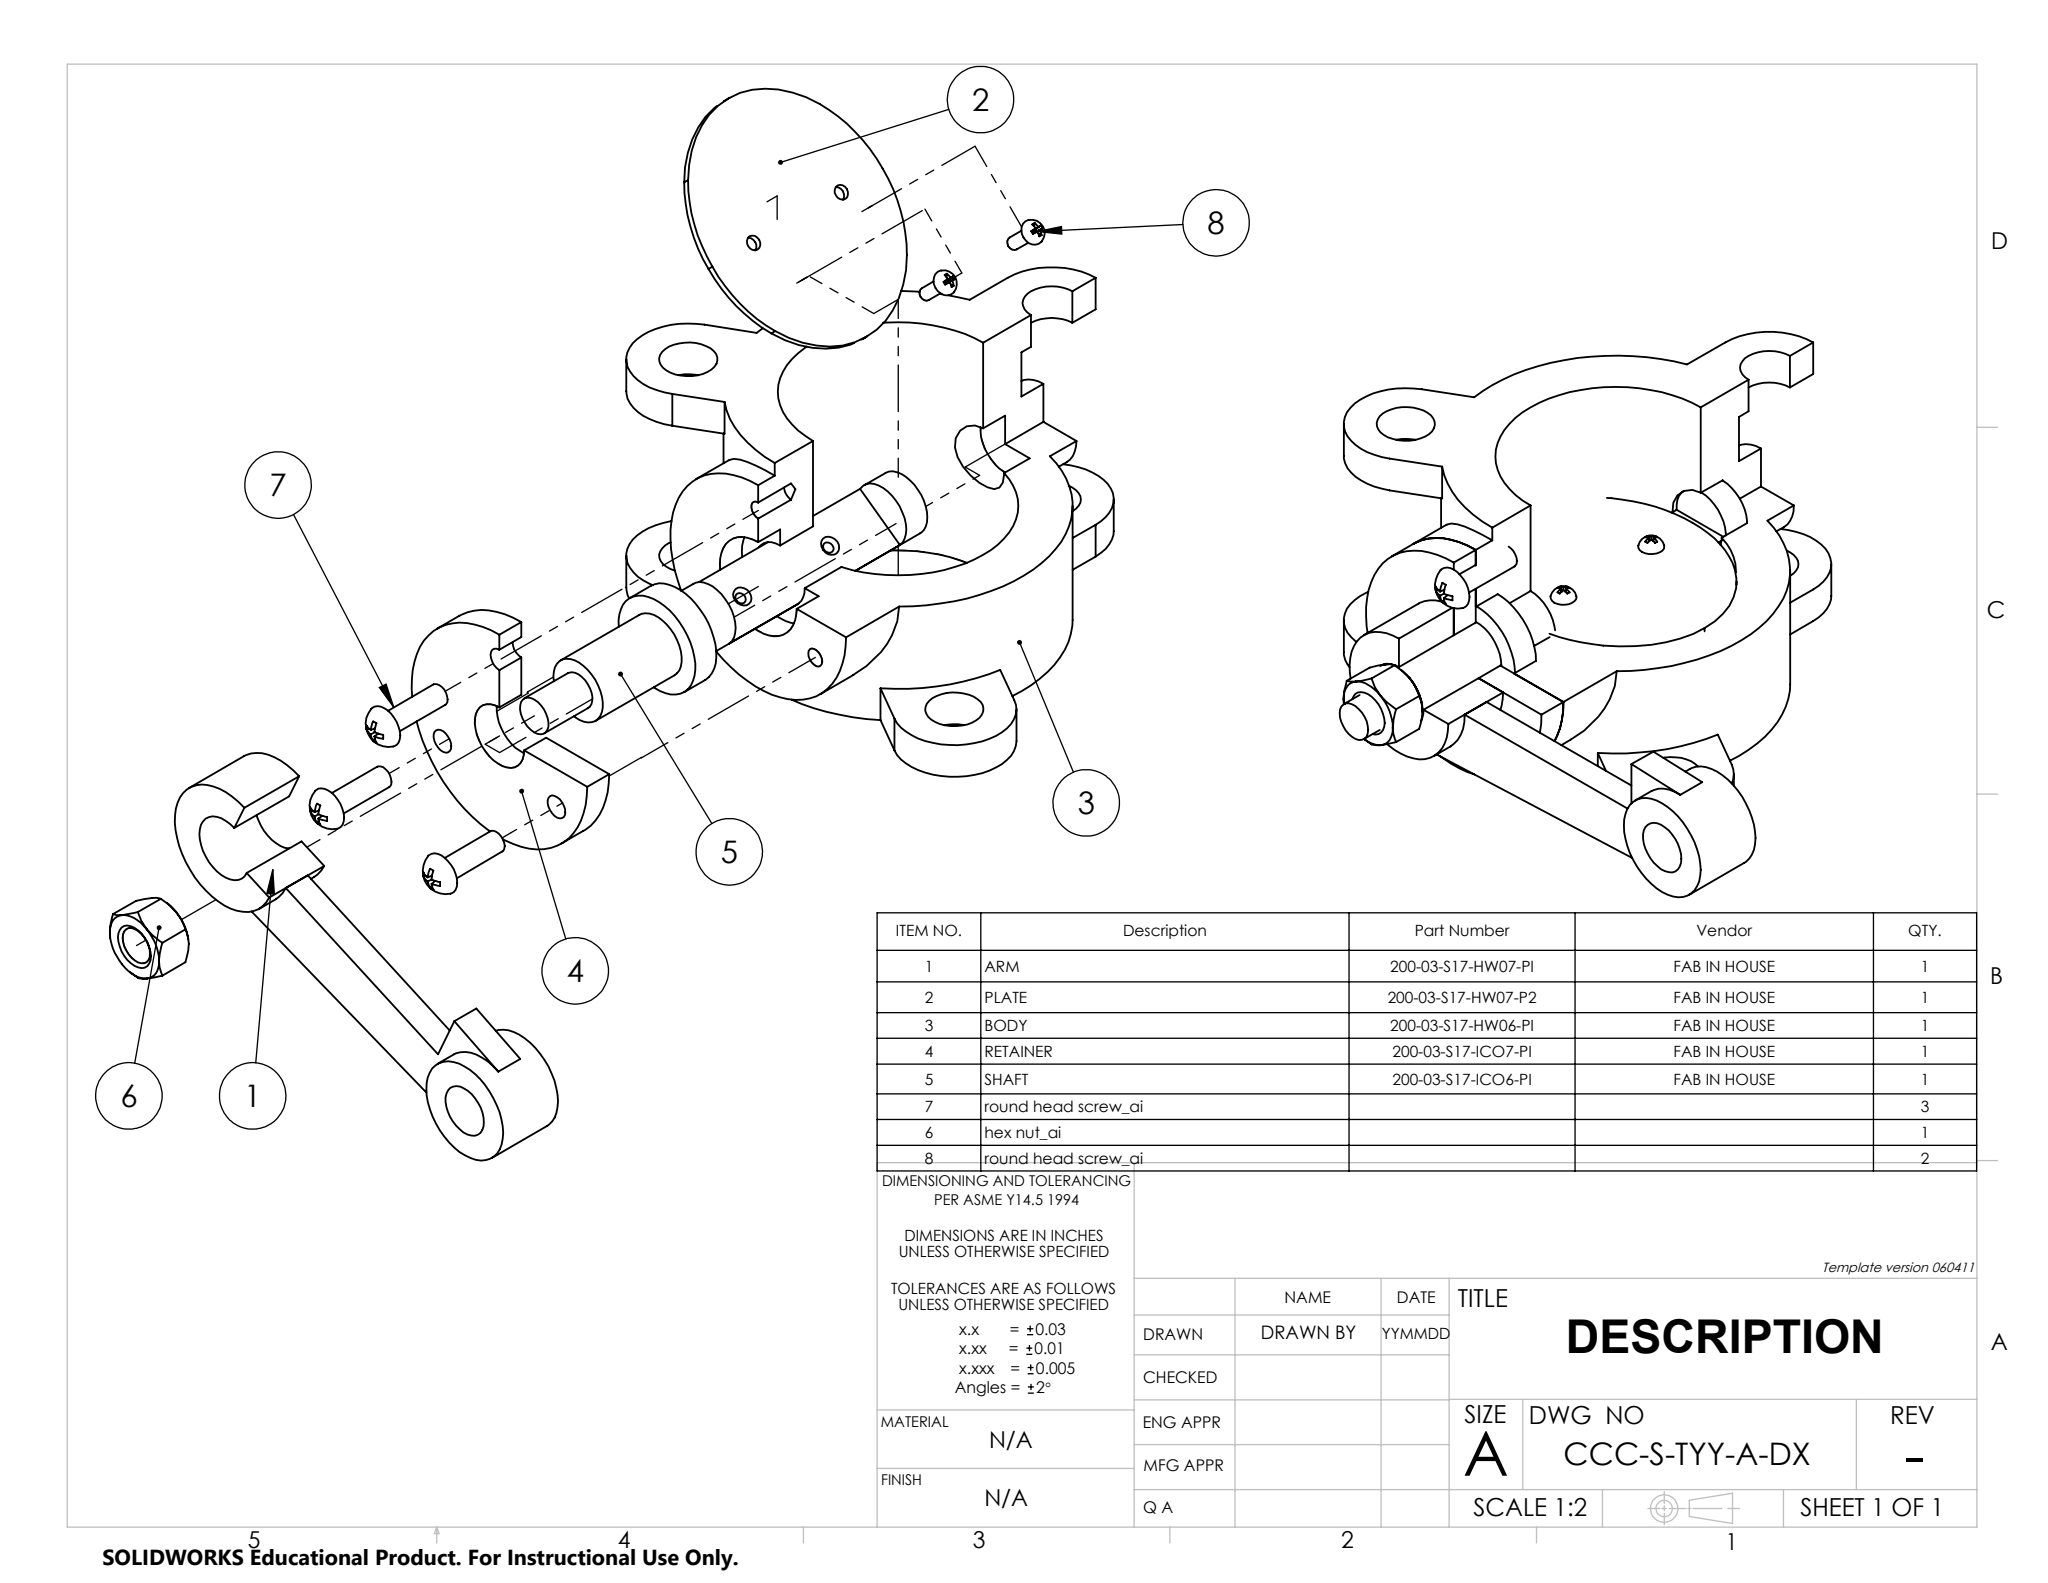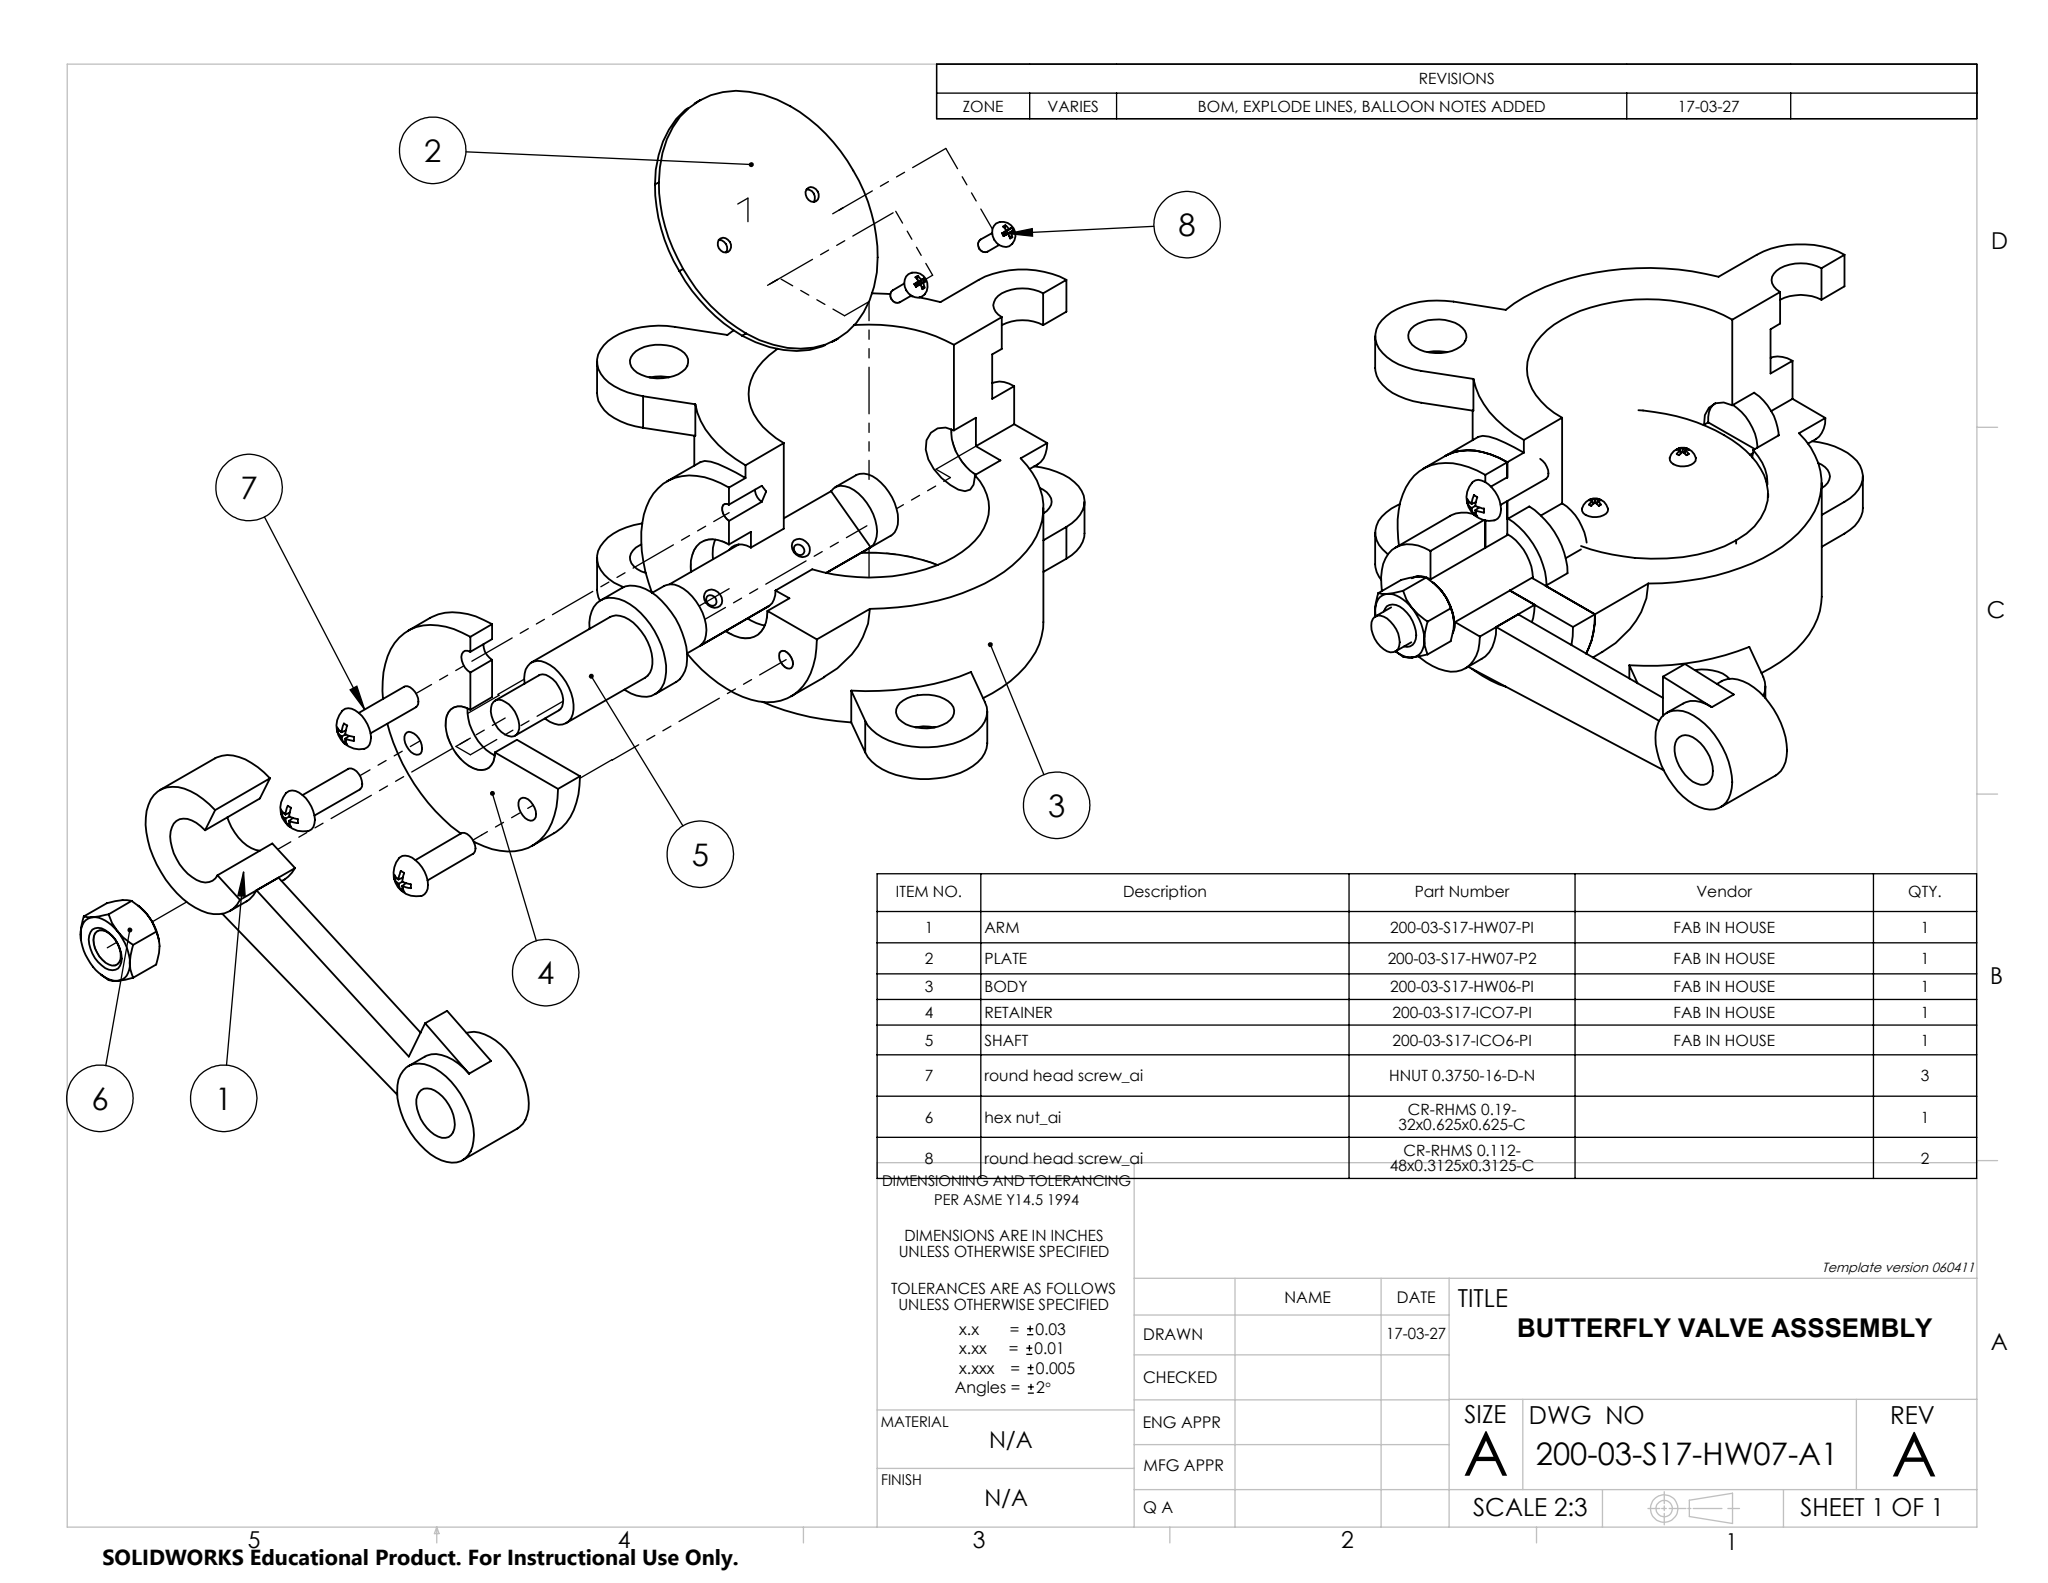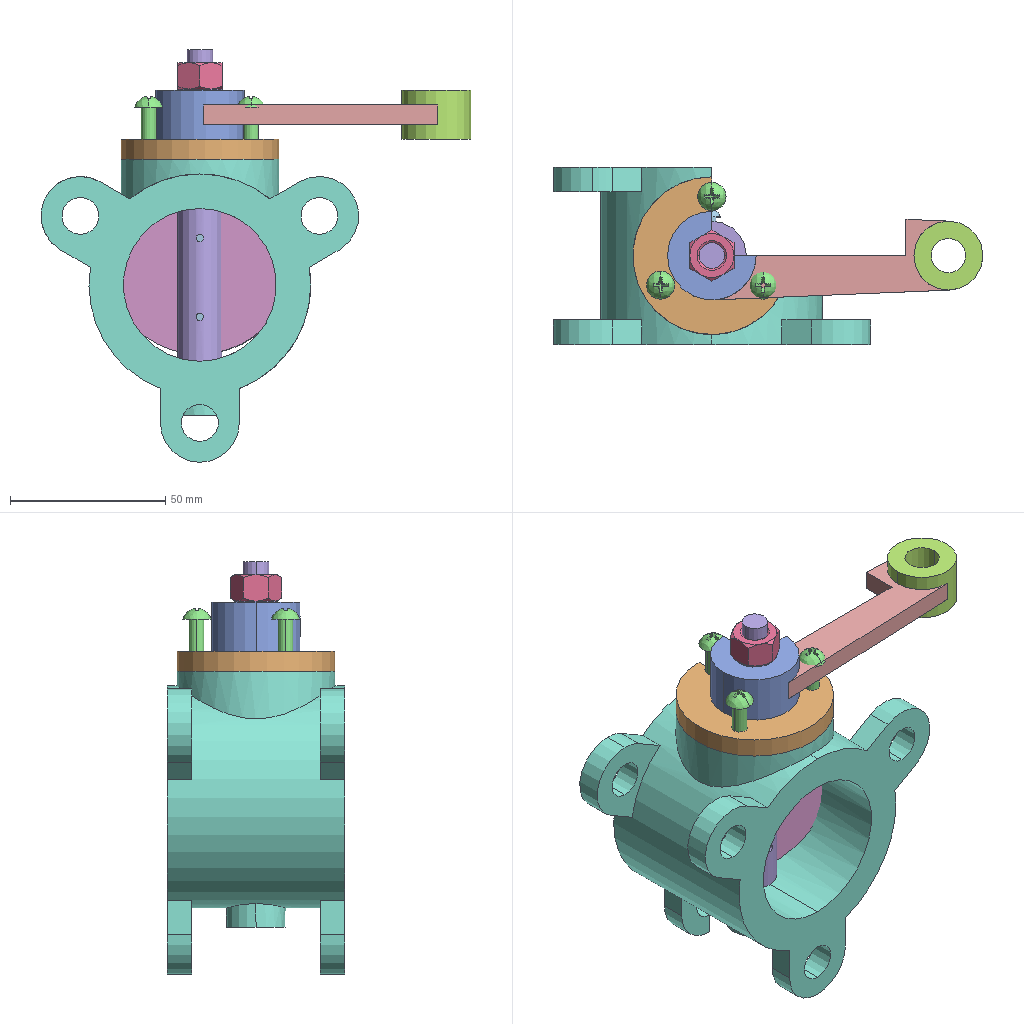Assembly | SolidWorks | 8 different items | 8 placed | box 138 x 57 x 133 mm
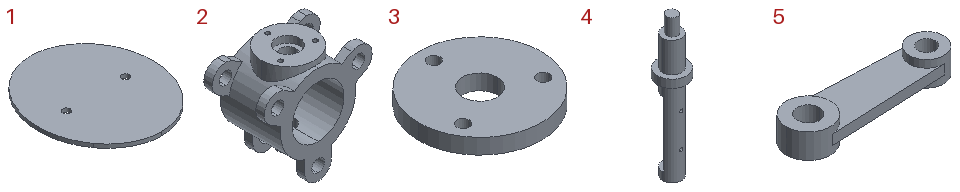Parts list (item | name | quantity | size | volume | features):
1 | - | x1 | 49.231 x 56.342 x 1.6 mm | 3464 mm3 | features Extrusion 1, ICE 1
2 | - | x1 | 102.39 x 57.15 x 97.638 mm | 149520 mm3 | features ICE 5, CirPattern 1, Extrusion 1, HoleWzd 1, MirrorPattern 1, RefAxis 1
3 | - | x1 | 50.8 x 50.8 x 6.35 mm | 11453 mm3 | features Extrusion 1, ICE 1
4 | - | x1 | 22.225 x 22.225 x 106.629 mm | 12564 mm3 | features ICE 6, HoleWzd 2, Extrusion 1, RefAxis 1
5 | - | x1 | 101.6 x 28.575 x 15.875 mm | 21274 mm3 | features ICE 2, Extrusion 1
6 | hex nut_ai | x1 | - | - | -
7 | round head screw_ai | x1 | - | - | -
8 | round head screw_ai1 | x1 | - | - | -
Mates (type | each side: item.copy, entity, surface, feature):
Coincident | 2.1 edge | 4.1 edge
Coincident | 2.1 edge | 3.1 edge
Coincident | 5.1 edge | 3.1 edge
Concentric | 1.1 edge | 4.1 edge | 2 times
Coincident | 1.1 face plane Boss-Extrude1 | 4.1 face plane Cut-Extrude3
Concentric | 5.1 edge | 3.1 edge